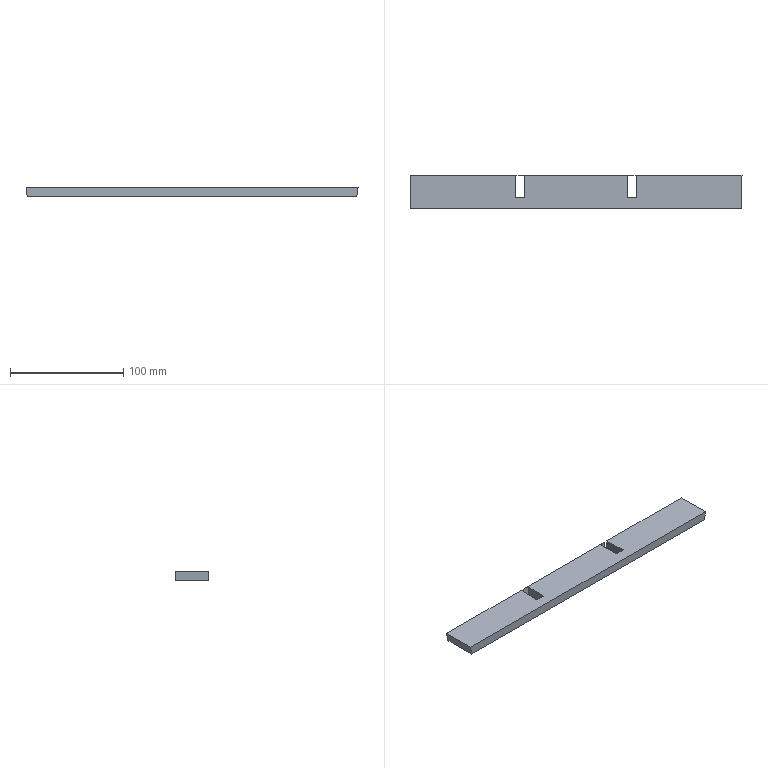Part | SolidWorks | features BaseBody 1 | 1 solid | 16 faces | box 293.1 x 30 x 8 mm | volume 66811 mm3 | plane 16
STEP:
#1=CARTESIAN_POINT('',(50.601,14.398,0.));
#2=VERTEX_POINT('',#1);
#3=CARTESIAN_POINT('',(50.887,15.,8.));
#4=VERTEX_POINT('',#3);
#5=CARTESIAN_POINT('',(50.601,14.398,0.));
#6=DIRECTION('',(0.0356,0.07493,0.9966));
#7=VECTOR('',#6,1000.);
#8=LINE('',#5,#7);
#9=EDGE_CURVE('',#2,#4,#8,.T.);
#10=ORIENTED_EDGE('',*,*,#9,.F.);
#11=CARTESIAN_POINT('',(-50.601,14.398,0.));
#12=VERTEX_POINT('',#11);
#13=CARTESIAN_POINT('',(0.,14.398,0.));
#14=DIRECTION('',(1.,0.,0.));
#15=VECTOR('',#14,1000.);
#16=LINE('',#13,#15);
#17=EDGE_CURVE('',#12,#2,#16,.T.);
#18=ORIENTED_EDGE('',*,*,#17,.F.);
#19=CARTESIAN_POINT('',(-50.887,15.,8.));
#20=VERTEX_POINT('',#19);
#21=CARTESIAN_POINT('',(-50.887,15.,8.));
#22=DIRECTION('',(0.0356,-0.07493,-0.9966));
#23=VECTOR('',#22,1000.);
#24=LINE('',#21,#23);
#25=EDGE_CURVE('',#20,#12,#24,.T.);
#26=ORIENTED_EDGE('',*,*,#25,.F.);
#27=CARTESIAN_POINT('',(0.,15.,8.));
#28=DIRECTION('',(-1.,0.,0.));
#29=VECTOR('',#28,1000.);
#30=LINE('',#27,#29);
#31=EDGE_CURVE('',#4,#20,#30,.T.);
#32=ORIENTED_EDGE('',*,*,#31,.F.);
#33=EDGE_LOOP('',(#10,#18,#26,#32));
#34=FACE_OUTER_BOUND('',#33,.T.);
#35=CARTESIAN_POINT('',(-51.498,15.,8.));
#36=DIRECTION('',(0.,-0.9972,0.07498));
#37=DIRECTION('',(0.,-0.07498,-0.9972));
#38=AXIS2_PLACEMENT_3D('',#35,#36,#37);
#39=PLANE('',#38);
#40=ADVANCED_FACE('',(#34),#39,.F.);
#41=CARTESIAN_POINT('',(45.305,14.835,8.));
#42=VERTEX_POINT('',#41);
#43=CARTESIAN_POINT('',(50.887,15.,8.));
#44=DIRECTION('',(-0.9996,-0.02956,0.));
#45=VECTOR('',#44,1000.);
#46=LINE('',#43,#45);
#47=EDGE_CURVE('',#4,#42,#46,.T.);
#48=ORIENTED_EDGE('',*,*,#47,.F.);
#49=ORIENTED_EDGE('',*,*,#31,.T.);
#50=CARTESIAN_POINT('',(-45.305,14.835,8.));
#51=VERTEX_POINT('',#50);
#52=CARTESIAN_POINT('',(-45.305,14.835,8.));
#53=DIRECTION('',(-0.9996,0.02956,0.));
#54=VECTOR('',#53,1000.);
#55=LINE('',#52,#54);
#56=EDGE_CURVE('',#51,#20,#55,.T.);
#57=ORIENTED_EDGE('',*,*,#56,.F.);
#58=CARTESIAN_POINT('',(-45.829,-5.213,8.));
#59=VERTEX_POINT('',#58);
#60=CARTESIAN_POINT('',(-45.829,-5.213,8.));
#61=DIRECTION('',(0.02613,0.9997,-0.000000001));
#62=VECTOR('',#61,1000.);
#63=LINE('',#60,#62);
#64=EDGE_CURVE('',#59,#51,#63,.T.);
#65=ORIENTED_EDGE('',*,*,#64,.F.);
#66=CARTESIAN_POINT('',(-53.834,-4.976,8.));
#67=VERTEX_POINT('',#66);
#68=CARTESIAN_POINT('',(-53.834,-4.976,8.));
#69=DIRECTION('',(0.9996,-0.02956,0.));
#70=VECTOR('',#69,1000.);
#71=LINE('',#68,#70);
#72=EDGE_CURVE('',#67,#59,#71,.T.);
#73=ORIENTED_EDGE('',*,*,#72,.F.);
#74=CARTESIAN_POINT('',(-53.312,15.,8.));
#75=VERTEX_POINT('',#74);
#76=CARTESIAN_POINT('',(-53.312,15.,8.));
#77=DIRECTION('',(-0.02613,-0.9997,0.));
#78=VECTOR('',#77,1000.);
#79=LINE('',#76,#78);
#80=EDGE_CURVE('',#75,#67,#79,.T.);
#81=ORIENTED_EDGE('',*,*,#80,.F.);
#82=CARTESIAN_POINT('',(-146.55,15.,8.));
#83=VERTEX_POINT('',#82);
#84=CARTESIAN_POINT('',(0.,15.,8.));
#85=DIRECTION('',(1.,0.,0.));
#86=VECTOR('',#85,1000.);
#87=LINE('',#84,#86);
#88=EDGE_CURVE('',#83,#75,#87,.T.);
#89=ORIENTED_EDGE('',*,*,#88,.F.);
#90=CARTESIAN_POINT('',(-146.55,-15.,8.));
#91=VERTEX_POINT('',#90);
#92=CARTESIAN_POINT('',(-146.55,0.,8.));
#93=DIRECTION('',(0.,1.,0.));
#94=VECTOR('',#93,1000.);
#95=LINE('',#92,#94);
#96=EDGE_CURVE('',#91,#83,#95,.T.);
#97=ORIENTED_EDGE('',*,*,#96,.F.);
#98=CARTESIAN_POINT('',(146.55,-15.,8.));
#99=VERTEX_POINT('',#98);
#100=CARTESIAN_POINT('',(0.,-15.,8.));
#101=DIRECTION('',(-1.,0.,0.));
#102=VECTOR('',#101,1000.);
#103=LINE('',#100,#102);
#104=EDGE_CURVE('',#99,#91,#103,.T.);
#105=ORIENTED_EDGE('',*,*,#104,.F.);
#106=CARTESIAN_POINT('',(146.55,15.,8.));
#107=VERTEX_POINT('',#106);
#108=CARTESIAN_POINT('',(146.55,0.,8.));
#109=DIRECTION('',(0.,-1.,0.));
#110=VECTOR('',#109,1000.);
#111=LINE('',#108,#110);
#112=EDGE_CURVE('',#107,#99,#111,.T.);
#113=ORIENTED_EDGE('',*,*,#112,.F.);
#114=CARTESIAN_POINT('',(53.312,15.,8.));
#115=VERTEX_POINT('',#114);
#116=CARTESIAN_POINT('',(0.,15.,8.));
#117=DIRECTION('',(1.,0.,0.));
#118=VECTOR('',#117,1000.);
#119=LINE('',#116,#118);
#120=EDGE_CURVE('',#115,#107,#119,.T.);
#121=ORIENTED_EDGE('',*,*,#120,.F.);
#122=CARTESIAN_POINT('',(53.834,-4.976,8.));
#123=VERTEX_POINT('',#122);
#124=CARTESIAN_POINT('',(53.834,-4.976,8.));
#125=DIRECTION('',(-0.02613,0.9997,0.));
#126=VECTOR('',#125,1000.);
#127=LINE('',#124,#126);
#128=EDGE_CURVE('',#123,#115,#127,.T.);
#129=ORIENTED_EDGE('',*,*,#128,.F.);
#130=CARTESIAN_POINT('',(45.829,-5.213,8.));
#131=VERTEX_POINT('',#130);
#132=CARTESIAN_POINT('',(45.829,-5.213,8.));
#133=DIRECTION('',(0.9996,0.02956,0.));
#134=VECTOR('',#133,1000.);
#135=LINE('',#132,#134);
#136=EDGE_CURVE('',#131,#123,#135,.T.);
#137=ORIENTED_EDGE('',*,*,#136,.F.);
#138=CARTESIAN_POINT('',(45.305,14.835,8.));
#139=DIRECTION('',(0.02613,-0.9997,0.000000001));
#140=VECTOR('',#139,1000.);
#141=LINE('',#138,#140);
#142=EDGE_CURVE('',#42,#131,#141,.T.);
#143=ORIENTED_EDGE('',*,*,#142,.F.);
#144=EDGE_LOOP('',(#48,#49,#57,#65,#73,#81,#89,#97,#105,#113,#121,#129,#137,#143));
#145=FACE_OUTER_BOUND('',#144,.T.);
#146=CARTESIAN_POINT('',(146.55,-15.,8.));
#147=DIRECTION('',(0.,0.,-1.));
#148=DIRECTION('',(-1.,0.,0.));
#149=AXIS2_PLACEMENT_3D('',#146,#147,#148);
#150=PLANE('',#149);
#151=ADVANCED_FACE('',(#145),#150,.F.);
#152=CARTESIAN_POINT('',(44.95,14.231,0.));
#153=VERTEX_POINT('',#152);
#154=CARTESIAN_POINT('',(50.601,14.398,0.));
#155=DIRECTION('',(-0.9996,-0.02956,0.));
#156=VECTOR('',#155,1000.);
#157=LINE('',#154,#156);
#158=EDGE_CURVE('',#2,#153,#157,.T.);
#159=ORIENTED_EDGE('',*,*,#158,.F.);
#160=ORIENTED_EDGE('',*,*,#9,.T.);
#161=ORIENTED_EDGE('',*,*,#47,.T.);
#162=CARTESIAN_POINT('',(44.95,14.231,0.000000007));
#163=DIRECTION('',(0.04418,0.07516,0.9962));
#164=VECTOR('',#163,1000.);
#165=LINE('',#162,#164);
#166=EDGE_CURVE('',#153,#42,#165,.T.);
#167=ORIENTED_EDGE('',*,*,#166,.F.);
#168=EDGE_LOOP('',(#159,#160,#161,#167));
#169=FACE_OUTER_BOUND('',#168,.T.);
#170=CARTESIAN_POINT('',(44.915,14.227,-0.048));
#171=DIRECTION('',(-0.02948,0.9968,-0.0739));
#172=DIRECTION('',(0.,0.07393,0.9973));
#173=AXIS2_PLACEMENT_3D('',#170,#171,#172);
#174=PLANE('',#173);
#175=ADVANCED_FACE('',(#169),#174,.F.);
#176=CARTESIAN_POINT('',(-44.95,14.231,0.));
#177=VERTEX_POINT('',#176);
#178=CARTESIAN_POINT('',(-44.95,14.231,0.));
#179=DIRECTION('',(-0.9996,0.02956,0.));
#180=VECTOR('',#179,1000.);
#181=LINE('',#178,#180);
#182=EDGE_CURVE('',#177,#12,#181,.T.);
#183=ORIENTED_EDGE('',*,*,#182,.T.);
#184=ORIENTED_EDGE('',*,*,#17,.T.);
#185=ORIENTED_EDGE('',*,*,#158,.T.);
#186=CARTESIAN_POINT('',(45.474,-5.817,0.));
#187=VERTEX_POINT('',#186);
#188=CARTESIAN_POINT('',(44.95,14.231,0.));
#189=DIRECTION('',(0.02613,-0.9997,0.));
#190=VECTOR('',#189,1000.);
#191=LINE('',#188,#190);
#192=EDGE_CURVE('',#153,#187,#191,.T.);
#193=ORIENTED_EDGE('',*,*,#192,.T.);
#194=CARTESIAN_POINT('',(53.48,-5.58,0.));
#195=VERTEX_POINT('',#194);
#196=CARTESIAN_POINT('',(45.474,-5.817,0.));
#197=DIRECTION('',(0.9996,0.02956,0.));
#198=VECTOR('',#197,1000.);
#199=LINE('',#196,#198);
#200=EDGE_CURVE('',#187,#195,#199,.T.);
#201=ORIENTED_EDGE('',*,*,#200,.T.);
#202=CARTESIAN_POINT('',(52.957,14.398,0.));
#203=VERTEX_POINT('',#202);
#204=CARTESIAN_POINT('',(53.48,-5.58,0.));
#205=DIRECTION('',(-0.02613,0.9997,0.));
#206=VECTOR('',#205,1000.);
#207=LINE('',#204,#206);
#208=EDGE_CURVE('',#195,#203,#207,.T.);
#209=ORIENTED_EDGE('',*,*,#208,.T.);
#210=CARTESIAN_POINT('',(145.454,14.398,0.));
#211=VERTEX_POINT('',#210);
#212=CARTESIAN_POINT('',(0.,14.398,0.));
#213=DIRECTION('',(1.,0.,0.));
#214=VECTOR('',#213,1000.);
#215=LINE('',#212,#214);
#216=EDGE_CURVE('',#203,#211,#215,.T.);
#217=ORIENTED_EDGE('',*,*,#216,.T.);
#218=CARTESIAN_POINT('',(145.454,-15.,0.));
#219=VERTEX_POINT('',#218);
#220=CARTESIAN_POINT('',(145.454,-0.3008,0.));
#221=DIRECTION('',(0.,-1.,0.));
#222=VECTOR('',#221,1000.);
#223=LINE('',#220,#222);
#224=EDGE_CURVE('',#211,#219,#223,.T.);
#225=ORIENTED_EDGE('',*,*,#224,.T.);
#226=CARTESIAN_POINT('',(-145.454,-15.,0.));
#227=VERTEX_POINT('',#226);
#228=CARTESIAN_POINT('',(0.,-15.,0.));
#229=DIRECTION('',(-1.,0.,0.));
#230=VECTOR('',#229,1000.);
#231=LINE('',#228,#230);
#232=EDGE_CURVE('',#219,#227,#231,.T.);
#233=ORIENTED_EDGE('',*,*,#232,.T.);
#234=CARTESIAN_POINT('',(-145.454,14.398,0.));
#235=VERTEX_POINT('',#234);
#236=CARTESIAN_POINT('',(-145.454,-0.3008,0.));
#237=DIRECTION('',(0.,1.,0.));
#238=VECTOR('',#237,1000.);
#239=LINE('',#236,#238);
#240=EDGE_CURVE('',#227,#235,#239,.T.);
#241=ORIENTED_EDGE('',*,*,#240,.T.);
#242=CARTESIAN_POINT('',(-52.957,14.398,0.));
#243=VERTEX_POINT('',#242);
#244=CARTESIAN_POINT('',(0.,14.398,0.));
#245=DIRECTION('',(1.,0.,0.));
#246=VECTOR('',#245,1000.);
#247=LINE('',#244,#246);
#248=EDGE_CURVE('',#235,#243,#247,.T.);
#249=ORIENTED_EDGE('',*,*,#248,.T.);
#250=CARTESIAN_POINT('',(-53.48,-5.58,0.));
#251=VERTEX_POINT('',#250);
#252=CARTESIAN_POINT('',(-52.957,14.398,0.));
#253=DIRECTION('',(-0.02613,-0.9997,0.));
#254=VECTOR('',#253,1000.);
#255=LINE('',#252,#254);
#256=EDGE_CURVE('',#243,#251,#255,.T.);
#257=ORIENTED_EDGE('',*,*,#256,.T.);
#258=CARTESIAN_POINT('',(-45.474,-5.817,0.));
#259=VERTEX_POINT('',#258);
#260=CARTESIAN_POINT('',(-53.48,-5.58,0.));
#261=DIRECTION('',(0.9996,-0.02956,0.));
#262=VECTOR('',#261,1000.);
#263=LINE('',#260,#262);
#264=EDGE_CURVE('',#251,#259,#263,.T.);
#265=ORIENTED_EDGE('',*,*,#264,.T.);
#266=CARTESIAN_POINT('',(-45.474,-5.817,0.));
#267=DIRECTION('',(0.02613,0.9997,0.));
#268=VECTOR('',#267,1000.);
#269=LINE('',#266,#268);
#270=EDGE_CURVE('',#259,#177,#269,.T.);
#271=ORIENTED_EDGE('',*,*,#270,.T.);
#272=EDGE_LOOP('',(#183,#184,#185,#193,#201,#209,#217,#225,#233,#241,#249,#257,#265,#271));
#273=FACE_OUTER_BOUND('',#272,.T.);
#274=CARTESIAN_POINT('',(145.454,-15.,0.));
#275=DIRECTION('',(0.,0.,-1.));
#276=DIRECTION('',(-1.,0.,0.));
#277=AXIS2_PLACEMENT_3D('',#274,#275,#276);
#278=PLANE('',#277);
#279=ADVANCED_FACE('',(#273),#278,.T.);
#280=ORIENTED_EDGE('',*,*,#182,.F.);
#281=CARTESIAN_POINT('',(-45.305,14.835,8.));
#282=DIRECTION('',(0.04418,-0.07516,-0.9962));
#283=VECTOR('',#282,1000.);
#284=LINE('',#281,#283);
#285=EDGE_CURVE('',#51,#177,#284,.T.);
#286=ORIENTED_EDGE('',*,*,#285,.F.);
#287=ORIENTED_EDGE('',*,*,#56,.T.);
#288=ORIENTED_EDGE('',*,*,#25,.T.);
#289=EDGE_LOOP('',(#280,#286,#287,#288));
#290=FACE_OUTER_BOUND('',#289,.T.);
#291=CARTESIAN_POINT('',(-50.923,14.403,-0.0611));
#292=DIRECTION('',(0.02948,0.9968,-0.0739));
#293=DIRECTION('',(0.,0.07393,0.9973));
#294=AXIS2_PLACEMENT_3D('',#291,#292,#293);
#295=PLANE('',#294);
#296=ADVANCED_FACE('',(#290),#295,.F.);
#297=ORIENTED_EDGE('',*,*,#192,.F.);
#298=ORIENTED_EDGE('',*,*,#166,.T.);
#299=ORIENTED_EDGE('',*,*,#142,.T.);
#300=CARTESIAN_POINT('',(45.474,-5.817,0.000000003));
#301=DIRECTION('',(0.04418,0.07516,0.9962));
#302=VECTOR('',#301,1000.);
#303=LINE('',#300,#302);
#304=EDGE_CURVE('',#187,#131,#303,.T.);
#305=ORIENTED_EDGE('',*,*,#304,.F.);
#306=EDGE_LOOP('',(#297,#298,#299,#305));
#307=FACE_OUTER_BOUND('',#306,.T.);
#308=CARTESIAN_POINT('',(45.474,-5.941,-0.07251));
#309=DIRECTION('',(-0.9986,-0.0261,0.04626));
#310=DIRECTION('',(0.04627,0.,0.9989));
#311=AXIS2_PLACEMENT_3D('',#308,#309,#310);
#312=PLANE('',#311);
#313=ADVANCED_FACE('',(#307),#312,.F.);
#314=ORIENTED_EDGE('',*,*,#270,.F.);
#315=CARTESIAN_POINT('',(-45.829,-5.213,8.));
#316=DIRECTION('',(0.04418,-0.07516,-0.9962));
#317=VECTOR('',#316,1000.);
#318=LINE('',#315,#317);
#319=EDGE_CURVE('',#59,#259,#318,.T.);
#320=ORIENTED_EDGE('',*,*,#319,.F.);
#321=ORIENTED_EDGE('',*,*,#64,.T.);
#322=ORIENTED_EDGE('',*,*,#285,.T.);
#323=EDGE_LOOP('',(#314,#320,#321,#322));
#324=FACE_OUTER_BOUND('',#323,.T.);
#325=CARTESIAN_POINT('',(-45.85,-5.941,8.047));
#326=DIRECTION('',(0.9986,-0.0261,0.04626));
#327=DIRECTION('',(0.04627,0.,-0.9989));
#328=AXIS2_PLACEMENT_3D('',#325,#326,#327);
#329=PLANE('',#328);
#330=ADVANCED_FACE('',(#324),#329,.F.);
#331=ORIENTED_EDGE('',*,*,#264,.F.);
#332=CARTESIAN_POINT('',(-53.834,-4.976,8.));
#333=DIRECTION('',(0.04418,-0.07516,-0.9962));
#334=VECTOR('',#333,1000.);
#335=LINE('',#332,#334);
#336=EDGE_CURVE('',#67,#251,#335,.T.);
#337=ORIENTED_EDGE('',*,*,#336,.F.);
#338=ORIENTED_EDGE('',*,*,#72,.T.);
#339=ORIENTED_EDGE('',*,*,#319,.T.);
#340=EDGE_LOOP('',(#331,#337,#338,#339));
#341=FACE_OUTER_BOUND('',#340,.T.);
#342=CARTESIAN_POINT('',(-53.884,-4.971,8.048));
#343=DIRECTION('',(-0.02948,-0.9968,0.0739));
#344=DIRECTION('',(0.,-0.07393,-0.9973));
#345=AXIS2_PLACEMENT_3D('',#342,#343,#344);
#346=PLANE('',#345);
#347=ADVANCED_FACE('',(#341),#346,.F.);
#348=ORIENTED_EDGE('',*,*,#256,.F.);
#349=CARTESIAN_POINT('',(-53.312,15.,8.));
#350=DIRECTION('',(0.04419,-0.07491,-0.9962));
#351=VECTOR('',#350,1000.);
#352=LINE('',#349,#351);
#353=EDGE_CURVE('',#75,#243,#352,.T.);
#354=ORIENTED_EDGE('',*,*,#353,.F.);
#355=ORIENTED_EDGE('',*,*,#80,.T.);
#356=ORIENTED_EDGE('',*,*,#336,.T.);
#357=EDGE_LOOP('',(#348,#354,#355,#356));
#358=FACE_OUTER_BOUND('',#357,.T.);
#359=CARTESIAN_POINT('',(-53.479,-5.704,-0.07242));
#360=DIRECTION('',(-0.9986,0.0261,-0.04626));
#361=DIRECTION('',(-0.04627,0.,0.9989));
#362=AXIS2_PLACEMENT_3D('',#359,#360,#361);
#363=PLANE('',#362);
#364=ADVANCED_FACE('',(#358),#363,.F.);
#365=ORIENTED_EDGE('',*,*,#353,.T.);
#366=ORIENTED_EDGE('',*,*,#248,.F.);
#367=CARTESIAN_POINT('',(-146.55,15.,8.));
#368=DIRECTION('',(0.1353,-0.07429,-0.988));
#369=VECTOR('',#368,1000.);
#370=LINE('',#367,#369);
#371=EDGE_CURVE('',#83,#235,#370,.T.);
#372=ORIENTED_EDGE('',*,*,#371,.F.);
#373=ORIENTED_EDGE('',*,*,#88,.T.);
#374=EDGE_LOOP('',(#365,#366,#372,#373));
#375=FACE_OUTER_BOUND('',#374,.T.);
#376=CARTESIAN_POINT('',(-147.112,15.,8.));
#377=DIRECTION('',(0.,-0.9972,0.07498));
#378=DIRECTION('',(0.,-0.07498,-0.9972));
#379=AXIS2_PLACEMENT_3D('',#376,#377,#378);
#380=PLANE('',#379);
#381=ADVANCED_FACE('',(#375),#380,.F.);
#382=CARTESIAN_POINT('',(-146.002,-15.,4.));
#383=DIRECTION('',(0.1357,0.,-0.9907));
#384=VECTOR('',#383,1000.);
#385=LINE('',#382,#384);
#386=EDGE_CURVE('',#91,#227,#385,.T.);
#387=ORIENTED_EDGE('',*,*,#386,.F.);
#388=ORIENTED_EDGE('',*,*,#96,.T.);
#389=ORIENTED_EDGE('',*,*,#371,.T.);
#390=ORIENTED_EDGE('',*,*,#240,.F.);
#391=EDGE_LOOP('',(#387,#388,#389,#390));
#392=FACE_OUTER_BOUND('',#391,.T.);
#393=CARTESIAN_POINT('',(-146.55,-15.,8.));
#394=DIRECTION('',(0.9907,0.,0.1357));
#395=DIRECTION('',(0.1357,0.,-0.9907));
#396=AXIS2_PLACEMENT_3D('',#393,#394,#395);
#397=PLANE('',#396);
#398=ADVANCED_FACE('',(#392),#397,.F.);
#399=CARTESIAN_POINT('',(145.454,-15.,0.));
#400=DIRECTION('',(-0.1357,0.,-0.9907));
#401=VECTOR('',#400,1000.);
#402=LINE('',#399,#401);
#403=EDGE_CURVE('',#99,#219,#402,.T.);
#404=ORIENTED_EDGE('',*,*,#403,.F.);
#405=ORIENTED_EDGE('',*,*,#104,.T.);
#406=ORIENTED_EDGE('',*,*,#386,.T.);
#407=ORIENTED_EDGE('',*,*,#232,.F.);
#408=EDGE_LOOP('',(#404,#405,#406,#407));
#409=FACE_OUTER_BOUND('',#408,.T.);
#410=CARTESIAN_POINT('',(148.309,-15.,0.));
#411=DIRECTION('',(0.,1.,0.));
#412=DIRECTION('',(-1.,0.,0.));
#413=AXIS2_PLACEMENT_3D('',#410,#411,#412);
#414=PLANE('',#413);
#415=ADVANCED_FACE('',(#409),#414,.F.);
#416=CARTESIAN_POINT('',(146.55,15.,8.));
#417=DIRECTION('',(-0.1353,-0.07429,-0.988));
#418=VECTOR('',#417,1000.);
#419=LINE('',#416,#418);
#420=EDGE_CURVE('',#107,#211,#419,.T.);
#421=ORIENTED_EDGE('',*,*,#420,.F.);
#422=ORIENTED_EDGE('',*,*,#112,.T.);
#423=ORIENTED_EDGE('',*,*,#403,.T.);
#424=ORIENTED_EDGE('',*,*,#224,.F.);
#425=EDGE_LOOP('',(#421,#422,#423,#424));
#426=FACE_OUTER_BOUND('',#425,.T.);
#427=CARTESIAN_POINT('',(145.454,-15.,0.));
#428=DIRECTION('',(-0.9907,0.,0.1357));
#429=DIRECTION('',(0.1357,0.,0.9907));
#430=AXIS2_PLACEMENT_3D('',#427,#428,#429);
#431=PLANE('',#430);
#432=ADVANCED_FACE('',(#426),#431,.F.);
#433=CARTESIAN_POINT('',(53.312,15.,8.));
#434=DIRECTION('',(-0.04419,-0.07491,-0.9962));
#435=VECTOR('',#434,1000.);
#436=LINE('',#433,#435);
#437=EDGE_CURVE('',#115,#203,#436,.T.);
#438=ORIENTED_EDGE('',*,*,#437,.F.);
#439=ORIENTED_EDGE('',*,*,#120,.T.);
#440=ORIENTED_EDGE('',*,*,#420,.T.);
#441=ORIENTED_EDGE('',*,*,#216,.F.);
#442=EDGE_LOOP('',(#438,#439,#440,#441));
#443=FACE_OUTER_BOUND('',#442,.T.);
#444=CARTESIAN_POINT('',(52.396,15.,8.));
#445=DIRECTION('',(0.,-0.9972,0.07498));
#446=DIRECTION('',(0.,-0.07498,-0.9972));
#447=AXIS2_PLACEMENT_3D('',#444,#445,#446);
#448=PLANE('',#447);
#449=ADVANCED_FACE('',(#443),#448,.F.);
#450=ORIENTED_EDGE('',*,*,#208,.F.);
#451=CARTESIAN_POINT('',(53.834,-4.976,8.));
#452=DIRECTION('',(-0.04418,-0.07516,-0.9962));
#453=VECTOR('',#452,1000.);
#454=LINE('',#451,#453);
#455=EDGE_CURVE('',#123,#195,#454,.T.);
#456=ORIENTED_EDGE('',*,*,#455,.F.);
#457=ORIENTED_EDGE('',*,*,#128,.T.);
#458=ORIENTED_EDGE('',*,*,#437,.T.);
#459=EDGE_LOOP('',(#450,#456,#457,#458));
#460=FACE_OUTER_BOUND('',#459,.T.);
#461=CARTESIAN_POINT('',(53.855,-5.704,8.047));
#462=DIRECTION('',(0.9986,0.0261,-0.04626));
#463=DIRECTION('',(-0.04627,0.,-0.9989));
#464=AXIS2_PLACEMENT_3D('',#461,#462,#463);
#465=PLANE('',#464);
#466=ADVANCED_FACE('',(#460),#465,.F.);
#467=ORIENTED_EDGE('',*,*,#200,.F.);
#468=ORIENTED_EDGE('',*,*,#304,.T.);
#469=ORIENTED_EDGE('',*,*,#136,.T.);
#470=ORIENTED_EDGE('',*,*,#455,.T.);
#471=EDGE_LOOP('',(#467,#468,#469,#470));
#472=FACE_OUTER_BOUND('',#471,.T.);
#473=CARTESIAN_POINT('',(45.424,-5.22,8.066));
#474=DIRECTION('',(0.02948,-0.9968,0.0739));
#475=DIRECTION('',(0.,-0.07393,-0.9973));
#476=AXIS2_PLACEMENT_3D('',#473,#474,#475);
#477=PLANE('',#476);
#478=ADVANCED_FACE('',(#472),#477,.F.);
#479=CLOSED_SHELL('',(#40,#151,#175,#279,#296,#313,#330,#347,#364,#381,#398,#415,#432,#449,#466,#478));
#480=MANIFOLD_SOLID_BREP('',#479);
#481=CARTESIAN_POINT('',(0.,0.,0.));
#482=DIRECTION('',(0.,0.,1.));
#483=DIRECTION('',(1.,0.,0.));
#484=AXIS2_PLACEMENT_3D('',#481,#482,#483);
#485=(LENGTH_UNIT()NAMED_UNIT(*)SI_UNIT(.MILLI.,.METRE.));
#486=UNCERTAINTY_MEASURE_WITH_UNIT(LENGTH_MEASURE(0.00001),#485,'','');
#487=(NAMED_UNIT(*)PLANE_ANGLE_UNIT()SI_UNIT($,.RADIAN.));
#488=(NAMED_UNIT(*)SI_UNIT($,.STERADIAN.)SOLID_ANGLE_UNIT());
#489=(GEOMETRIC_REPRESENTATION_CONTEXT(3)GLOBAL_UNCERTAINTY_ASSIGNED_CONTEXT((#486))GLOBAL_UNIT_ASSIGNED_CONTEXT((#485,#487,#488))REPRESENTATION_CONTEXT('',''));
#490=ADVANCED_BREP_SHAPE_REPRESENTATION('',(#480,#484),#489);